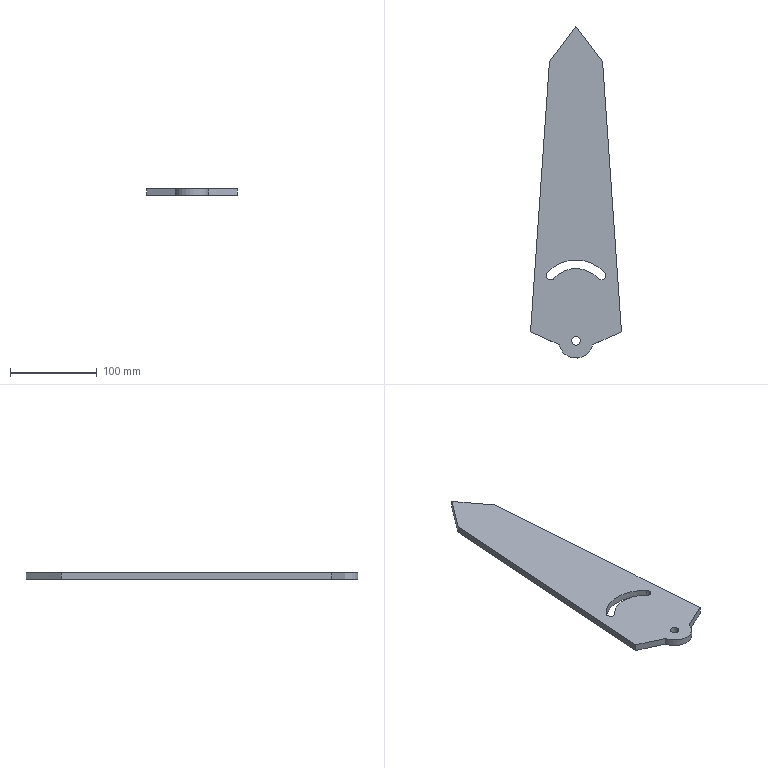Part | SolidWorks | features Cut 1, Extrusion 1 | 1 solid | 16 faces | box 105.1 x 383.944 x 8 mm | volume 223880 mm3 | cylinder 8 | plane 8 | commonest cylinder face diameters 10 x5 39.783 x1 68.646 x1 88.646 x1
STEP:
#1=CARTESIAN_POINT('',(34.597,1259.406,0.));
#2=VERTEX_POINT('',#1);
#3=CARTESIAN_POINT('',(33.346,1262.714,0.));
#4=VERTEX_POINT('',#3);
#5=CARTESIAN_POINT('',(29.597,1259.406,0.));
#6=DIRECTION('',(0.,0.,1.));
#7=DIRECTION('',(1.,0.,0.));
#8=AXIS2_PLACEMENT_3D('',#5,#6,#7);
#9=CIRCLE('',#8,5.);
#10=EDGE_CURVE('',#2,#4,#9,.T.);
#11=ORIENTED_EDGE('',*,*,#10,.F.);
#12=CARTESIAN_POINT('',(34.597,1259.406,8.));
#13=VERTEX_POINT('',#12);
#14=CARTESIAN_POINT('',(34.597,1259.406,-2.));
#15=DIRECTION('',(0.,0.,1.));
#16=VECTOR('',#15,1000.);
#17=LINE('',#14,#16);
#18=EDGE_CURVE('',#2,#13,#17,.T.);
#19=ORIENTED_EDGE('',*,*,#18,.T.);
#20=CARTESIAN_POINT('',(33.346,1262.714,8.));
#21=VERTEX_POINT('',#20);
#22=CARTESIAN_POINT('',(29.597,1259.406,8.));
#23=DIRECTION('',(0.,0.,1.));
#24=DIRECTION('',(1.,0.,0.));
#25=AXIS2_PLACEMENT_3D('',#22,#23,#24);
#26=CIRCLE('',#25,5.);
#27=EDGE_CURVE('',#13,#21,#26,.T.);
#28=ORIENTED_EDGE('',*,*,#27,.T.);
#29=CARTESIAN_POINT('',(33.346,1262.714,-2.));
#30=DIRECTION('',(0.,0.,1.));
#31=VECTOR('',#30,1000.);
#32=LINE('',#29,#31);
#33=EDGE_CURVE('',#4,#21,#32,.T.);
#34=ORIENTED_EDGE('',*,*,#33,.F.);
#35=EDGE_LOOP('',(#11,#19,#28,#34));
#36=FACE_OUTER_BOUND('',#35,.T.);
#37=CARTESIAN_POINT('',(29.597,1259.406,-2.));
#38=DIRECTION('',(0.,0.,1.));
#39=DIRECTION('',(1.,0.,0.));
#40=AXIS2_PLACEMENT_3D('',#37,#38,#39);
#41=CYLINDRICAL_SURFACE('',#40,5.);
#42=ADVANCED_FACE('',(#36),#41,.F.);
#43=CARTESIAN_POINT('',(-5.,1184.,8.));
#44=VERTEX_POINT('',#43);
#45=CARTESIAN_POINT('',(5.,1184.,8.));
#46=VERTEX_POINT('',#45);
#47=CARTESIAN_POINT('',(0.,1184.,8.));
#48=DIRECTION('',(0.,0.,1.));
#49=DIRECTION('',(1.,0.,0.));
#50=AXIS2_PLACEMENT_3D('',#47,#48,#49);
#51=CIRCLE('',#50,5.);
#52=EDGE_CURVE('',#44,#46,#51,.T.);
#53=ORIENTED_EDGE('',*,*,#52,.T.);
#54=CARTESIAN_POINT('',(5.,1184.,0.));
#55=VERTEX_POINT('',#54);
#56=CARTESIAN_POINT('',(5.,1184.,8.));
#57=DIRECTION('',(0.,0.,-1.));
#58=VECTOR('',#57,1000.);
#59=LINE('',#56,#58);
#60=EDGE_CURVE('',#46,#55,#59,.T.);
#61=ORIENTED_EDGE('',*,*,#60,.T.);
#62=CARTESIAN_POINT('',(-5.,1184.,0.));
#63=VERTEX_POINT('',#62);
#64=CARTESIAN_POINT('',(0.,1184.,0.));
#65=DIRECTION('',(0.,0.,1.));
#66=DIRECTION('',(1.,0.,0.));
#67=AXIS2_PLACEMENT_3D('',#64,#65,#66);
#68=CIRCLE('',#67,5.);
#69=EDGE_CURVE('',#63,#55,#68,.T.);
#70=ORIENTED_EDGE('',*,*,#69,.F.);
#71=CARTESIAN_POINT('',(-5.,1184.,8.));
#72=DIRECTION('',(0.,0.,-1.));
#73=VECTOR('',#72,1000.);
#74=LINE('',#71,#73);
#75=EDGE_CURVE('',#44,#63,#74,.T.);
#76=ORIENTED_EDGE('',*,*,#75,.F.);
#77=EDGE_LOOP('',(#53,#61,#70,#76));
#78=FACE_OUTER_BOUND('',#77,.T.);
#79=CARTESIAN_POINT('',(0.,1184.,8.));
#80=DIRECTION('',(0.,0.,-1.));
#81=DIRECTION('',(-1.,0.,0.));
#82=AXIS2_PLACEMENT_3D('',#79,#80,#81);
#83=CYLINDRICAL_SURFACE('',#82,5.);
#84=ADVANCED_FACE('',(#78),#83,.F.);
#85=CARTESIAN_POINT('',(-25.525,1256.21,8.));
#86=VERTEX_POINT('',#85);
#87=CARTESIAN_POINT('',(25.848,1256.098,8.));
#88=VERTEX_POINT('',#87);
#89=CARTESIAN_POINT('',(0.1114,1233.389,8.));
#90=DIRECTION('',(0.,0.,-1.));
#91=DIRECTION('',(1.,0.,0.));
#92=AXIS2_PLACEMENT_3D('',#89,#90,#91);
#93=CIRCLE('',#92,34.323);
#94=EDGE_CURVE('',#86,#88,#93,.T.);
#95=ORIENTED_EDGE('',*,*,#94,.F.);
#96=CARTESIAN_POINT('',(-32.995,1262.859,8.));
#97=VERTEX_POINT('',#96);
#98=CARTESIAN_POINT('',(-29.26,1259.535,8.));
#99=DIRECTION('',(0.,0.,1.));
#100=DIRECTION('',(1.,0.,0.));
#101=AXIS2_PLACEMENT_3D('',#98,#99,#100);
#102=CIRCLE('',#101,5.);
#103=EDGE_CURVE('',#97,#86,#102,.T.);
#104=ORIENTED_EDGE('',*,*,#103,.F.);
#105=CARTESIAN_POINT('',(0.1114,1233.389,8.));
#106=DIRECTION('',(0.,0.,-1.));
#107=DIRECTION('',(1.,0.,0.));
#108=AXIS2_PLACEMENT_3D('',#105,#106,#107);
#109=CIRCLE('',#108,44.323);
#110=EDGE_CURVE('',#97,#21,#109,.T.);
#111=ORIENTED_EDGE('',*,*,#110,.T.);
#112=ORIENTED_EDGE('',*,*,#27,.F.);
#113=CARTESIAN_POINT('',(29.597,1259.406,8.));
#114=DIRECTION('',(0.,0.,1.));
#115=DIRECTION('',(1.,0.,0.));
#116=AXIS2_PLACEMENT_3D('',#113,#114,#115);
#117=CIRCLE('',#116,5.);
#118=EDGE_CURVE('',#88,#13,#117,.T.);
#119=ORIENTED_EDGE('',*,*,#118,.F.);
#120=EDGE_LOOP('',(#95,#104,#111,#112,#119));
#121=FACE_BOUND('',#120,.T.);
#122=CARTESIAN_POINT('',(-52.439,1194.6,8.));
#123=VERTEX_POINT('',#122);
#124=CARTESIAN_POINT('',(-19.402,1179.614,8.));
#125=VERTEX_POINT('',#124);
#126=CARTESIAN_POINT('',(-52.439,1194.6,8.));
#127=DIRECTION('',(0.9107,-0.4131,0.));
#128=VECTOR('',#127,1000.);
#129=LINE('',#126,#128);
#130=EDGE_CURVE('',#123,#125,#129,.T.);
#131=ORIENTED_EDGE('',*,*,#130,.T.);
#132=CARTESIAN_POINT('',(19.376,1179.501,8.));
#133=VERTEX_POINT('',#132);
#134=CARTESIAN_POINT('',(0.,1184.,8.));
#135=DIRECTION('',(0.,0.,1.));
#136=DIRECTION('',(1.,0.,0.));
#137=AXIS2_PLACEMENT_3D('',#134,#135,#136);
#138=CIRCLE('',#137,19.891);
#139=EDGE_CURVE('',#125,#133,#138,.T.);
#140=ORIENTED_EDGE('',*,*,#139,.T.);
#141=CARTESIAN_POINT('',(52.661,1194.6,8.));
#142=VERTEX_POINT('',#141);
#143=CARTESIAN_POINT('',(52.661,1194.6,8.));
#144=DIRECTION('',(0.9107,0.4131,0.));
#145=VECTOR('',#144,1000.);
#146=LINE('',#143,#145);
#147=EDGE_CURVE('',#133,#142,#146,.T.);
#148=ORIENTED_EDGE('',*,*,#147,.T.);
#149=CARTESIAN_POINT('',(30.793,1507.337,8.));
#150=VERTEX_POINT('',#149);
#151=CARTESIAN_POINT('',(52.661,1194.6,8.));
#152=DIRECTION('',(-0.06976,0.9976,0.));
#153=VECTOR('',#152,1000.);
#154=LINE('',#151,#153);
#155=EDGE_CURVE('',#142,#150,#154,.T.);
#156=ORIENTED_EDGE('',*,*,#155,.T.);
#157=CARTESIAN_POINT('',(0.,1548.052,8.));
#158=VERTEX_POINT('',#157);
#159=CARTESIAN_POINT('',(0.,1548.052,8.));
#160=DIRECTION('',(-0.6032,0.7976,0.));
#161=VECTOR('',#160,1000.);
#162=LINE('',#159,#161);
#163=EDGE_CURVE('',#150,#158,#162,.T.);
#164=ORIENTED_EDGE('',*,*,#163,.T.);
#165=CARTESIAN_POINT('',(-30.57,1507.337,8.));
#166=VERTEX_POINT('',#165);
#167=CARTESIAN_POINT('',(0.,1548.052,8.));
#168=DIRECTION('',(-0.6004,-0.7997,0.));
#169=VECTOR('',#168,1000.);
#170=LINE('',#167,#169);
#171=EDGE_CURVE('',#158,#166,#170,.T.);
#172=ORIENTED_EDGE('',*,*,#171,.T.);
#173=CARTESIAN_POINT('',(-52.439,1194.6,8.));
#174=DIRECTION('',(-0.06976,-0.9976,0.));
#175=VECTOR('',#174,1000.);
#176=LINE('',#173,#175);
#177=EDGE_CURVE('',#166,#123,#176,.T.);
#178=ORIENTED_EDGE('',*,*,#177,.T.);
#179=EDGE_LOOP('',(#131,#140,#148,#156,#164,#172,#178));
#180=FACE_OUTER_BOUND('',#179,.T.);
#181=ORIENTED_EDGE('',*,*,#52,.F.);
#182=CARTESIAN_POINT('',(0.,1184.,8.));
#183=DIRECTION('',(0.,0.,1.));
#184=DIRECTION('',(1.,0.,0.));
#185=AXIS2_PLACEMENT_3D('',#182,#183,#184);
#186=CIRCLE('',#185,5.);
#187=EDGE_CURVE('',#46,#44,#186,.T.);
#188=ORIENTED_EDGE('',*,*,#187,.F.);
#189=EDGE_LOOP('',(#181,#188));
#190=FACE_BOUND('',#189,.T.);
#191=CARTESIAN_POINT('',(0.,1184.,8.));
#192=DIRECTION('',(0.,0.,1.));
#193=DIRECTION('',(1.,0.,0.));
#194=AXIS2_PLACEMENT_3D('',#191,#192,#193);
#195=PLANE('',#194);
#196=ADVANCED_FACE('',(#121,#180,#190),#195,.T.);
#197=CARTESIAN_POINT('',(-32.995,1262.859,0.));
#198=VERTEX_POINT('',#197);
#199=CARTESIAN_POINT('',(-25.525,1256.21,0.));
#200=VERTEX_POINT('',#199);
#201=CARTESIAN_POINT('',(-29.26,1259.535,0.));
#202=DIRECTION('',(0.,0.,1.));
#203=DIRECTION('',(1.,0.,0.));
#204=AXIS2_PLACEMENT_3D('',#201,#202,#203);
#205=CIRCLE('',#204,5.);
#206=EDGE_CURVE('',#198,#200,#205,.T.);
#207=ORIENTED_EDGE('',*,*,#206,.T.);
#208=CARTESIAN_POINT('',(25.848,1256.098,0.));
#209=VERTEX_POINT('',#208);
#210=CARTESIAN_POINT('',(0.1114,1233.389,0.));
#211=DIRECTION('',(0.,0.,-1.));
#212=DIRECTION('',(1.,0.,0.));
#213=AXIS2_PLACEMENT_3D('',#210,#211,#212);
#214=CIRCLE('',#213,34.323);
#215=EDGE_CURVE('',#200,#209,#214,.T.);
#216=ORIENTED_EDGE('',*,*,#215,.T.);
#217=CARTESIAN_POINT('',(29.597,1259.406,0.));
#218=DIRECTION('',(0.,0.,1.));
#219=DIRECTION('',(1.,0.,0.));
#220=AXIS2_PLACEMENT_3D('',#217,#218,#219);
#221=CIRCLE('',#220,5.);
#222=EDGE_CURVE('',#209,#2,#221,.T.);
#223=ORIENTED_EDGE('',*,*,#222,.T.);
#224=ORIENTED_EDGE('',*,*,#10,.T.);
#225=CARTESIAN_POINT('',(0.1114,1233.389,0.));
#226=DIRECTION('',(0.,0.,-1.));
#227=DIRECTION('',(1.,0.,0.));
#228=AXIS2_PLACEMENT_3D('',#225,#226,#227);
#229=CIRCLE('',#228,44.323);
#230=EDGE_CURVE('',#198,#4,#229,.T.);
#231=ORIENTED_EDGE('',*,*,#230,.F.);
#232=EDGE_LOOP('',(#207,#216,#223,#224,#231));
#233=FACE_BOUND('',#232,.T.);
#234=CARTESIAN_POINT('',(-52.439,1194.6,0.));
#235=VERTEX_POINT('',#234);
#236=CARTESIAN_POINT('',(-19.402,1179.614,0.));
#237=VERTEX_POINT('',#236);
#238=CARTESIAN_POINT('',(-52.439,1194.6,0.));
#239=DIRECTION('',(0.9107,-0.4131,0.));
#240=VECTOR('',#239,1000.);
#241=LINE('',#238,#240);
#242=EDGE_CURVE('',#235,#237,#241,.T.);
#243=ORIENTED_EDGE('',*,*,#242,.F.);
#244=CARTESIAN_POINT('',(-30.57,1507.337,0.));
#245=VERTEX_POINT('',#244);
#246=CARTESIAN_POINT('',(-52.439,1194.6,0.));
#247=DIRECTION('',(-0.06976,-0.9976,0.));
#248=VECTOR('',#247,1000.);
#249=LINE('',#246,#248);
#250=EDGE_CURVE('',#245,#235,#249,.T.);
#251=ORIENTED_EDGE('',*,*,#250,.F.);
#252=CARTESIAN_POINT('',(0.,1548.052,0.));
#253=VERTEX_POINT('',#252);
#254=CARTESIAN_POINT('',(0.,1548.052,0.));
#255=DIRECTION('',(-0.6004,-0.7997,0.));
#256=VECTOR('',#255,1000.);
#257=LINE('',#254,#256);
#258=EDGE_CURVE('',#253,#245,#257,.T.);
#259=ORIENTED_EDGE('',*,*,#258,.F.);
#260=CARTESIAN_POINT('',(30.793,1507.337,0.));
#261=VERTEX_POINT('',#260);
#262=CARTESIAN_POINT('',(0.,1548.052,0.));
#263=DIRECTION('',(-0.6032,0.7976,0.));
#264=VECTOR('',#263,1000.);
#265=LINE('',#262,#264);
#266=EDGE_CURVE('',#261,#253,#265,.T.);
#267=ORIENTED_EDGE('',*,*,#266,.F.);
#268=CARTESIAN_POINT('',(52.661,1194.6,0.));
#269=VERTEX_POINT('',#268);
#270=CARTESIAN_POINT('',(52.661,1194.6,0.));
#271=DIRECTION('',(-0.06976,0.9976,0.));
#272=VECTOR('',#271,1000.);
#273=LINE('',#270,#272);
#274=EDGE_CURVE('',#269,#261,#273,.T.);
#275=ORIENTED_EDGE('',*,*,#274,.F.);
#276=CARTESIAN_POINT('',(19.376,1179.501,0.));
#277=VERTEX_POINT('',#276);
#278=CARTESIAN_POINT('',(52.661,1194.6,0.));
#279=DIRECTION('',(0.9107,0.4131,0.));
#280=VECTOR('',#279,1000.);
#281=LINE('',#278,#280);
#282=EDGE_CURVE('',#277,#269,#281,.T.);
#283=ORIENTED_EDGE('',*,*,#282,.F.);
#284=CARTESIAN_POINT('',(0.,1184.,0.));
#285=DIRECTION('',(0.,0.,1.));
#286=DIRECTION('',(1.,0.,0.));
#287=AXIS2_PLACEMENT_3D('',#284,#285,#286);
#288=CIRCLE('',#287,19.891);
#289=EDGE_CURVE('',#237,#277,#288,.T.);
#290=ORIENTED_EDGE('',*,*,#289,.F.);
#291=EDGE_LOOP('',(#243,#251,#259,#267,#275,#283,#290));
#292=FACE_OUTER_BOUND('',#291,.T.);
#293=ORIENTED_EDGE('',*,*,#69,.T.);
#294=CARTESIAN_POINT('',(0.,1184.,0.));
#295=DIRECTION('',(0.,0.,1.));
#296=DIRECTION('',(1.,0.,0.));
#297=AXIS2_PLACEMENT_3D('',#294,#295,#296);
#298=CIRCLE('',#297,5.);
#299=EDGE_CURVE('',#55,#63,#298,.T.);
#300=ORIENTED_EDGE('',*,*,#299,.T.);
#301=EDGE_LOOP('',(#293,#300));
#302=FACE_BOUND('',#301,.T.);
#303=CARTESIAN_POINT('',(0.,1184.,0.));
#304=DIRECTION('',(0.,0.,1.));
#305=DIRECTION('',(1.,0.,0.));
#306=AXIS2_PLACEMENT_3D('',#303,#304,#305);
#307=PLANE('',#306);
#308=ADVANCED_FACE('',(#233,#292,#302),#307,.F.);
#309=ORIENTED_EDGE('',*,*,#242,.T.);
#310=CARTESIAN_POINT('',(-19.402,1179.614,8.));
#311=DIRECTION('',(0.,0.,-1.));
#312=VECTOR('',#311,1000.);
#313=LINE('',#310,#312);
#314=EDGE_CURVE('',#125,#237,#313,.T.);
#315=ORIENTED_EDGE('',*,*,#314,.F.);
#316=ORIENTED_EDGE('',*,*,#130,.F.);
#317=CARTESIAN_POINT('',(-52.439,1194.6,8.));
#318=DIRECTION('',(0.,0.,-1.));
#319=VECTOR('',#318,1000.);
#320=LINE('',#317,#319);
#321=EDGE_CURVE('',#123,#235,#320,.T.);
#322=ORIENTED_EDGE('',*,*,#321,.T.);
#323=EDGE_LOOP('',(#309,#315,#316,#322));
#324=FACE_OUTER_BOUND('',#323,.T.);
#325=CARTESIAN_POINT('',(-52.439,1194.6,8.));
#326=DIRECTION('',(0.4131,0.9107,0.));
#327=DIRECTION('',(-0.9107,0.4131,0.));
#328=AXIS2_PLACEMENT_3D('',#325,#326,#327);
#329=PLANE('',#328);
#330=ADVANCED_FACE('',(#324),#329,.F.);
#331=ORIENTED_EDGE('',*,*,#289,.T.);
#332=CARTESIAN_POINT('',(19.376,1179.501,8.));
#333=DIRECTION('',(0.,0.,-1.));
#334=VECTOR('',#333,1000.);
#335=LINE('',#332,#334);
#336=EDGE_CURVE('',#133,#277,#335,.T.);
#337=ORIENTED_EDGE('',*,*,#336,.F.);
#338=ORIENTED_EDGE('',*,*,#139,.F.);
#339=ORIENTED_EDGE('',*,*,#314,.T.);
#340=EDGE_LOOP('',(#331,#337,#338,#339));
#341=FACE_OUTER_BOUND('',#340,.T.);
#342=CARTESIAN_POINT('',(0.,1184.,8.));
#343=DIRECTION('',(0.,0.,-1.));
#344=DIRECTION('',(-1.,0.,0.));
#345=AXIS2_PLACEMENT_3D('',#342,#343,#344);
#346=CYLINDRICAL_SURFACE('',#345,19.891);
#347=ADVANCED_FACE('',(#341),#346,.T.);
#348=ORIENTED_EDGE('',*,*,#282,.T.);
#349=CARTESIAN_POINT('',(52.661,1194.6,8.));
#350=DIRECTION('',(0.,0.,-1.));
#351=VECTOR('',#350,1000.);
#352=LINE('',#349,#351);
#353=EDGE_CURVE('',#142,#269,#352,.T.);
#354=ORIENTED_EDGE('',*,*,#353,.F.);
#355=ORIENTED_EDGE('',*,*,#147,.F.);
#356=ORIENTED_EDGE('',*,*,#336,.T.);
#357=EDGE_LOOP('',(#348,#354,#355,#356));
#358=FACE_OUTER_BOUND('',#357,.T.);
#359=CARTESIAN_POINT('',(52.661,1194.6,8.));
#360=DIRECTION('',(-0.4131,0.9107,0.));
#361=DIRECTION('',(-0.9107,-0.4131,0.));
#362=AXIS2_PLACEMENT_3D('',#359,#360,#361);
#363=PLANE('',#362);
#364=ADVANCED_FACE('',(#358),#363,.F.);
#365=ORIENTED_EDGE('',*,*,#274,.T.);
#366=CARTESIAN_POINT('',(30.793,1507.337,8.));
#367=DIRECTION('',(0.,0.,-1.));
#368=VECTOR('',#367,1000.);
#369=LINE('',#366,#368);
#370=EDGE_CURVE('',#150,#261,#369,.T.);
#371=ORIENTED_EDGE('',*,*,#370,.F.);
#372=ORIENTED_EDGE('',*,*,#155,.F.);
#373=ORIENTED_EDGE('',*,*,#353,.T.);
#374=EDGE_LOOP('',(#365,#371,#372,#373));
#375=FACE_OUTER_BOUND('',#374,.T.);
#376=CARTESIAN_POINT('',(52.661,1194.6,8.));
#377=DIRECTION('',(-0.9976,-0.06976,0.));
#378=DIRECTION('',(0.06976,-0.9976,0.));
#379=AXIS2_PLACEMENT_3D('',#376,#377,#378);
#380=PLANE('',#379);
#381=ADVANCED_FACE('',(#375),#380,.F.);
#382=ORIENTED_EDGE('',*,*,#266,.T.);
#383=CARTESIAN_POINT('',(0.,1548.052,8.));
#384=DIRECTION('',(0.,0.,-1.));
#385=VECTOR('',#384,1000.);
#386=LINE('',#383,#385);
#387=EDGE_CURVE('',#158,#253,#386,.T.);
#388=ORIENTED_EDGE('',*,*,#387,.F.);
#389=ORIENTED_EDGE('',*,*,#163,.F.);
#390=ORIENTED_EDGE('',*,*,#370,.T.);
#391=EDGE_LOOP('',(#382,#388,#389,#390));
#392=FACE_OUTER_BOUND('',#391,.T.);
#393=CARTESIAN_POINT('',(0.,1548.052,8.));
#394=DIRECTION('',(-0.7976,-0.6032,0.));
#395=DIRECTION('',(0.6032,-0.7976,0.));
#396=AXIS2_PLACEMENT_3D('',#393,#394,#395);
#397=PLANE('',#396);
#398=ADVANCED_FACE('',(#392),#397,.F.);
#399=ORIENTED_EDGE('',*,*,#258,.T.);
#400=CARTESIAN_POINT('',(-30.57,1507.337,8.));
#401=DIRECTION('',(0.,0.,-1.));
#402=VECTOR('',#401,1000.);
#403=LINE('',#400,#402);
#404=EDGE_CURVE('',#166,#245,#403,.T.);
#405=ORIENTED_EDGE('',*,*,#404,.F.);
#406=ORIENTED_EDGE('',*,*,#171,.F.);
#407=ORIENTED_EDGE('',*,*,#387,.T.);
#408=EDGE_LOOP('',(#399,#405,#406,#407));
#409=FACE_OUTER_BOUND('',#408,.T.);
#410=CARTESIAN_POINT('',(0.,1548.052,8.));
#411=DIRECTION('',(0.7997,-0.6004,0.));
#412=DIRECTION('',(0.6004,0.7997,0.));
#413=AXIS2_PLACEMENT_3D('',#410,#411,#412);
#414=PLANE('',#413);
#415=ADVANCED_FACE('',(#409),#414,.F.);
#416=ORIENTED_EDGE('',*,*,#250,.T.);
#417=ORIENTED_EDGE('',*,*,#321,.F.);
#418=ORIENTED_EDGE('',*,*,#177,.F.);
#419=ORIENTED_EDGE('',*,*,#404,.T.);
#420=EDGE_LOOP('',(#416,#417,#418,#419));
#421=FACE_OUTER_BOUND('',#420,.T.);
#422=CARTESIAN_POINT('',(-52.439,1194.6,8.));
#423=DIRECTION('',(0.9976,-0.06976,0.));
#424=DIRECTION('',(0.06976,0.9976,0.));
#425=AXIS2_PLACEMENT_3D('',#422,#423,#424);
#426=PLANE('',#425);
#427=ADVANCED_FACE('',(#421),#426,.F.);
#428=ORIENTED_EDGE('',*,*,#60,.F.);
#429=ORIENTED_EDGE('',*,*,#187,.T.);
#430=ORIENTED_EDGE('',*,*,#75,.T.);
#431=ORIENTED_EDGE('',*,*,#299,.F.);
#432=EDGE_LOOP('',(#428,#429,#430,#431));
#433=FACE_OUTER_BOUND('',#432,.T.);
#434=CARTESIAN_POINT('',(0.,1184.,8.));
#435=DIRECTION('',(0.,0.,-1.));
#436=DIRECTION('',(-1.,0.,0.));
#437=AXIS2_PLACEMENT_3D('',#434,#435,#436);
#438=CYLINDRICAL_SURFACE('',#437,5.);
#439=ADVANCED_FACE('',(#433),#438,.F.);
#440=CARTESIAN_POINT('',(-25.525,1256.21,-2.));
#441=DIRECTION('',(0.,0.,1.));
#442=VECTOR('',#441,1000.);
#443=LINE('',#440,#442);
#444=EDGE_CURVE('',#200,#86,#443,.T.);
#445=ORIENTED_EDGE('',*,*,#444,.T.);
#446=ORIENTED_EDGE('',*,*,#94,.T.);
#447=CARTESIAN_POINT('',(25.848,1256.098,-2.));
#448=DIRECTION('',(0.,0.,1.));
#449=VECTOR('',#448,1000.);
#450=LINE('',#447,#449);
#451=EDGE_CURVE('',#209,#88,#450,.T.);
#452=ORIENTED_EDGE('',*,*,#451,.F.);
#453=ORIENTED_EDGE('',*,*,#215,.F.);
#454=EDGE_LOOP('',(#445,#446,#452,#453));
#455=FACE_OUTER_BOUND('',#454,.T.);
#456=CARTESIAN_POINT('',(0.1114,1233.389,-2.));
#457=DIRECTION('',(0.,0.,1.));
#458=DIRECTION('',(1.,0.,0.));
#459=AXIS2_PLACEMENT_3D('',#456,#457,#458);
#460=CYLINDRICAL_SURFACE('',#459,34.323);
#461=ADVANCED_FACE('',(#455),#460,.T.);
#462=CARTESIAN_POINT('',(-32.995,1262.859,-2.));
#463=DIRECTION('',(0.,0.,1.));
#464=VECTOR('',#463,1000.);
#465=LINE('',#462,#464);
#466=EDGE_CURVE('',#198,#97,#465,.T.);
#467=ORIENTED_EDGE('',*,*,#466,.T.);
#468=ORIENTED_EDGE('',*,*,#103,.T.);
#469=ORIENTED_EDGE('',*,*,#444,.F.);
#470=ORIENTED_EDGE('',*,*,#206,.F.);
#471=EDGE_LOOP('',(#467,#468,#469,#470));
#472=FACE_OUTER_BOUND('',#471,.T.);
#473=CARTESIAN_POINT('',(-29.26,1259.535,-2.));
#474=DIRECTION('',(0.,0.,1.));
#475=DIRECTION('',(1.,0.,0.));
#476=AXIS2_PLACEMENT_3D('',#473,#474,#475);
#477=CYLINDRICAL_SURFACE('',#476,5.);
#478=ADVANCED_FACE('',(#472),#477,.F.);
#479=ORIENTED_EDGE('',*,*,#230,.T.);
#480=ORIENTED_EDGE('',*,*,#33,.T.);
#481=ORIENTED_EDGE('',*,*,#110,.F.);
#482=ORIENTED_EDGE('',*,*,#466,.F.);
#483=EDGE_LOOP('',(#479,#480,#481,#482));
#484=FACE_OUTER_BOUND('',#483,.T.);
#485=CARTESIAN_POINT('',(0.1114,1233.389,-2.));
#486=DIRECTION('',(0.,0.,1.));
#487=DIRECTION('',(1.,0.,0.));
#488=AXIS2_PLACEMENT_3D('',#485,#486,#487);
#489=CYLINDRICAL_SURFACE('',#488,44.323);
#490=ADVANCED_FACE('',(#484),#489,.F.);
#491=ORIENTED_EDGE('',*,*,#18,.F.);
#492=ORIENTED_EDGE('',*,*,#222,.F.);
#493=ORIENTED_EDGE('',*,*,#451,.T.);
#494=ORIENTED_EDGE('',*,*,#118,.T.);
#495=EDGE_LOOP('',(#491,#492,#493,#494));
#496=FACE_OUTER_BOUND('',#495,.T.);
#497=CARTESIAN_POINT('',(29.597,1259.406,-2.));
#498=DIRECTION('',(0.,0.,1.));
#499=DIRECTION('',(1.,0.,0.));
#500=AXIS2_PLACEMENT_3D('',#497,#498,#499);
#501=CYLINDRICAL_SURFACE('',#500,5.);
#502=ADVANCED_FACE('',(#496),#501,.F.);
#503=CLOSED_SHELL('',(#42,#84,#196,#308,#330,#347,#364,#381,#398,#415,#427,#439,#461,#478,#490,#502));
#504=MANIFOLD_SOLID_BREP('',#503);
#505=CARTESIAN_POINT('',(0.,0.,0.));
#506=DIRECTION('',(0.,0.,1.));
#507=DIRECTION('',(1.,0.,0.));
#508=AXIS2_PLACEMENT_3D('',#505,#506,#507);
#509=(LENGTH_UNIT()NAMED_UNIT(*)SI_UNIT(.MILLI.,.METRE.));
#510=UNCERTAINTY_MEASURE_WITH_UNIT(LENGTH_MEASURE(0.00001),#509,'','');
#511=(NAMED_UNIT(*)PLANE_ANGLE_UNIT()SI_UNIT($,.RADIAN.));
#512=(NAMED_UNIT(*)SI_UNIT($,.STERADIAN.)SOLID_ANGLE_UNIT());
#513=(GEOMETRIC_REPRESENTATION_CONTEXT(3)GLOBAL_UNCERTAINTY_ASSIGNED_CONTEXT((#510))GLOBAL_UNIT_ASSIGNED_CONTEXT((#509,#511,#512))REPRESENTATION_CONTEXT('',''));
#514=ADVANCED_BREP_SHAPE_REPRESENTATION('',(#504,#508),#513);